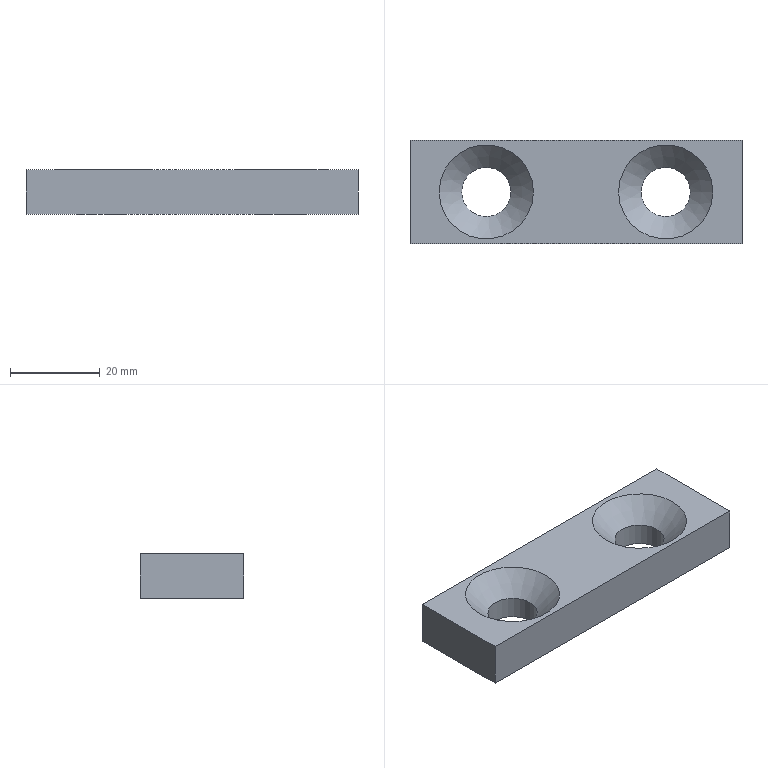Part | NX | features DATUM_CSYS 3, CSUNK_HOLE 2, HOLE PACKAGE 2, SKETCH 2, EXTRUDE 1, MIRROR_SET 1 | 1 solid | 10 faces | box 74 x 23 x 10 mm | volume 13994 mm3 | plane 6 | cylinder 2 | cone 2 | commonest cylinder face diameters 11 x2
STEP:
#1=CARTESIAN_POINT('',(-37.,-11.5,0.));
#2=VERTEX_POINT('',#1);
#3=CARTESIAN_POINT('',(37.,-11.5,0.));
#4=VERTEX_POINT('',#3);
#5=CARTESIAN_POINT('',(-37.,-11.5,0.));
#6=DIRECTION('',(1.,0.,0.));
#7=VECTOR('',#6,1000.);
#8=LINE('',#5,#7);
#9=EDGE_CURVE('',#2,#4,#8,.T.);
#10=ORIENTED_EDGE('',*,*,#9,.T.);
#11=CARTESIAN_POINT('',(37.,-11.5,10.));
#12=VERTEX_POINT('',#11);
#13=CARTESIAN_POINT('',(37.,-11.5,10.));
#14=DIRECTION('',(0.,0.,-1.));
#15=VECTOR('',#14,1000.);
#16=LINE('',#13,#15);
#17=EDGE_CURVE('',#12,#4,#16,.T.);
#18=ORIENTED_EDGE('',*,*,#17,.F.);
#19=CARTESIAN_POINT('',(-37.,-11.5,10.));
#20=VERTEX_POINT('',#19);
#21=CARTESIAN_POINT('',(-37.,-11.5,10.));
#22=DIRECTION('',(1.,0.,0.));
#23=VECTOR('',#22,1000.);
#24=LINE('',#21,#23);
#25=EDGE_CURVE('',#20,#12,#24,.T.);
#26=ORIENTED_EDGE('',*,*,#25,.F.);
#27=CARTESIAN_POINT('',(-37.,-11.5,10.));
#28=DIRECTION('',(0.,0.,-1.));
#29=VECTOR('',#28,1000.);
#30=LINE('',#27,#29);
#31=EDGE_CURVE('',#20,#2,#30,.T.);
#32=ORIENTED_EDGE('',*,*,#31,.T.);
#33=EDGE_LOOP('',(#10,#18,#26,#32));
#34=FACE_BOUND('',#33,.T.);
#35=CARTESIAN_POINT('',(-37.,-11.5,10.));
#36=DIRECTION('',(0.,1.,0.));
#37=DIRECTION('',(-1.,0.,0.));
#38=AXIS2_PLACEMENT_3D('',#35,#36,#37);
#39=PLANE('',#38);
#40=ADVANCED_FACE('',(#34),#39,.F.);
#41=CARTESIAN_POINT('',(37.,11.5,0.));
#42=VERTEX_POINT('',#41);
#43=CARTESIAN_POINT('',(37.,-11.5,0.));
#44=DIRECTION('',(0.,1.,0.));
#45=VECTOR('',#44,1000.);
#46=LINE('',#43,#45);
#47=EDGE_CURVE('',#4,#42,#46,.T.);
#48=ORIENTED_EDGE('',*,*,#47,.T.);
#49=CARTESIAN_POINT('',(37.,11.5,10.));
#50=VERTEX_POINT('',#49);
#51=CARTESIAN_POINT('',(37.,11.5,10.));
#52=DIRECTION('',(0.,0.,-1.));
#53=VECTOR('',#52,1000.);
#54=LINE('',#51,#53);
#55=EDGE_CURVE('',#50,#42,#54,.T.);
#56=ORIENTED_EDGE('',*,*,#55,.F.);
#57=CARTESIAN_POINT('',(37.,-11.5,10.));
#58=DIRECTION('',(0.,1.,0.));
#59=VECTOR('',#58,1000.);
#60=LINE('',#57,#59);
#61=EDGE_CURVE('',#12,#50,#60,.T.);
#62=ORIENTED_EDGE('',*,*,#61,.F.);
#63=ORIENTED_EDGE('',*,*,#17,.T.);
#64=EDGE_LOOP('',(#48,#56,#62,#63));
#65=FACE_BOUND('',#64,.T.);
#66=CARTESIAN_POINT('',(37.,-11.5,10.));
#67=DIRECTION('',(-1.,0.,0.));
#68=DIRECTION('',(0.,0.,1.));
#69=AXIS2_PLACEMENT_3D('',#66,#67,#68);
#70=PLANE('',#69);
#71=ADVANCED_FACE('',(#65),#70,.F.);
#72=CARTESIAN_POINT('',(-37.,11.5,0.));
#73=VERTEX_POINT('',#72);
#74=CARTESIAN_POINT('',(37.,11.5,0.));
#75=DIRECTION('',(-1.,0.,0.));
#76=VECTOR('',#75,1000.);
#77=LINE('',#74,#76);
#78=EDGE_CURVE('',#42,#73,#77,.T.);
#79=ORIENTED_EDGE('',*,*,#78,.T.);
#80=CARTESIAN_POINT('',(-37.,11.5,10.));
#81=VERTEX_POINT('',#80);
#82=CARTESIAN_POINT('',(-37.,11.5,10.));
#83=DIRECTION('',(0.,0.,-1.));
#84=VECTOR('',#83,1000.);
#85=LINE('',#82,#84);
#86=EDGE_CURVE('',#81,#73,#85,.T.);
#87=ORIENTED_EDGE('',*,*,#86,.F.);
#88=CARTESIAN_POINT('',(37.,11.5,10.));
#89=DIRECTION('',(-1.,0.,0.));
#90=VECTOR('',#89,1000.);
#91=LINE('',#88,#90);
#92=EDGE_CURVE('',#50,#81,#91,.T.);
#93=ORIENTED_EDGE('',*,*,#92,.F.);
#94=ORIENTED_EDGE('',*,*,#55,.T.);
#95=EDGE_LOOP('',(#79,#87,#93,#94));
#96=FACE_BOUND('',#95,.T.);
#97=CARTESIAN_POINT('',(37.,11.5,10.));
#98=DIRECTION('',(0.,-1.,0.));
#99=DIRECTION('',(1.,0.,0.));
#100=AXIS2_PLACEMENT_3D('',#97,#98,#99);
#101=PLANE('',#100);
#102=ADVANCED_FACE('',(#96),#101,.F.);
#103=CARTESIAN_POINT('',(-37.,11.5,0.));
#104=DIRECTION('',(0.,-1.,0.));
#105=VECTOR('',#104,1000.);
#106=LINE('',#103,#105);
#107=EDGE_CURVE('',#73,#2,#106,.T.);
#108=ORIENTED_EDGE('',*,*,#107,.T.);
#109=ORIENTED_EDGE('',*,*,#31,.F.);
#110=CARTESIAN_POINT('',(-37.,11.5,10.));
#111=DIRECTION('',(0.,-1.,0.));
#112=VECTOR('',#111,1000.);
#113=LINE('',#110,#112);
#114=EDGE_CURVE('',#81,#20,#113,.T.);
#115=ORIENTED_EDGE('',*,*,#114,.F.);
#116=ORIENTED_EDGE('',*,*,#86,.T.);
#117=EDGE_LOOP('',(#108,#109,#115,#116));
#118=FACE_BOUND('',#117,.T.);
#119=CARTESIAN_POINT('',(-37.,11.5,10.));
#120=DIRECTION('',(1.,0.,0.));
#121=DIRECTION('',(0.,0.,-1.));
#122=AXIS2_PLACEMENT_3D('',#119,#120,#121);
#123=PLANE('',#122);
#124=ADVANCED_FACE('',(#118),#123,.F.);
#125=CARTESIAN_POINT('',(30.5,0.,10.));
#126=VERTEX_POINT('',#125);
#127=CARTESIAN_POINT('',(20.,0.,10.));
#128=DIRECTION('',(0.,0.,1.));
#129=DIRECTION('',(1.,0.,0.));
#130=AXIS2_PLACEMENT_3D('',#127,#128,#129);
#131=CIRCLE('',#130,10.5);
#132=EDGE_CURVE('',#126,#126,#131,.T.);
#133=ORIENTED_EDGE('',*,*,#132,.F.);
#134=EDGE_LOOP('',(#133));
#135=FACE_BOUND('',#134,.T.);
#136=CARTESIAN_POINT('',(-30.5,0.,10.));
#137=VERTEX_POINT('',#136);
#138=CARTESIAN_POINT('',(-20.,0.,10.));
#139=DIRECTION('',(0.,0.,-1.));
#140=DIRECTION('',(-1.,0.,0.));
#141=AXIS2_PLACEMENT_3D('',#138,#139,#140);
#142=CIRCLE('',#141,10.5);
#143=EDGE_CURVE('',#137,#137,#142,.T.);
#144=ORIENTED_EDGE('',*,*,#143,.T.);
#145=EDGE_LOOP('',(#144));
#146=FACE_BOUND('',#145,.T.);
#147=ORIENTED_EDGE('',*,*,#25,.T.);
#148=ORIENTED_EDGE('',*,*,#61,.T.);
#149=ORIENTED_EDGE('',*,*,#92,.T.);
#150=ORIENTED_EDGE('',*,*,#114,.T.);
#151=EDGE_LOOP('',(#147,#148,#149,#150));
#152=FACE_BOUND('',#151,.T.);
#153=CARTESIAN_POINT('',(0.,0.,10.));
#154=DIRECTION('',(0.,0.,1.));
#155=DIRECTION('',(1.,0.,0.));
#156=AXIS2_PLACEMENT_3D('',#153,#154,#155);
#157=PLANE('',#156);
#158=ADVANCED_FACE('',(#135,#146,#152),#157,.T.);
#159=CARTESIAN_POINT('',(25.5,0.,0.));
#160=VERTEX_POINT('',#159);
#161=CARTESIAN_POINT('',(20.,0.,0.));
#162=DIRECTION('',(0.,0.,1.));
#163=DIRECTION('',(1.,0.,0.));
#164=AXIS2_PLACEMENT_3D('',#161,#162,#163);
#165=CIRCLE('',#164,5.5);
#166=EDGE_CURVE('',#160,#160,#165,.T.);
#167=ORIENTED_EDGE('',*,*,#166,.T.);
#168=EDGE_LOOP('',(#167));
#169=FACE_BOUND('',#168,.T.);
#170=CARTESIAN_POINT('',(-14.5,0.,0.));
#171=VERTEX_POINT('',#170);
#172=CARTESIAN_POINT('',(-20.,0.,0.));
#173=DIRECTION('',(0.,0.,1.));
#174=DIRECTION('',(1.,0.,0.));
#175=AXIS2_PLACEMENT_3D('',#172,#173,#174);
#176=CIRCLE('',#175,5.5);
#177=EDGE_CURVE('',#171,#171,#176,.T.);
#178=ORIENTED_EDGE('',*,*,#177,.T.);
#179=EDGE_LOOP('',(#178));
#180=FACE_BOUND('',#179,.T.);
#181=ORIENTED_EDGE('',*,*,#9,.F.);
#182=ORIENTED_EDGE('',*,*,#107,.F.);
#183=ORIENTED_EDGE('',*,*,#78,.F.);
#184=ORIENTED_EDGE('',*,*,#47,.F.);
#185=EDGE_LOOP('',(#181,#182,#183,#184));
#186=FACE_BOUND('',#185,.T.);
#187=CARTESIAN_POINT('',(0.,0.,0.));
#188=DIRECTION('',(0.,0.,1.));
#189=DIRECTION('',(1.,0.,0.));
#190=AXIS2_PLACEMENT_3D('',#187,#188,#189);
#191=PLANE('',#190);
#192=ADVANCED_FACE('',(#169,#180,#186),#191,.F.);
#193=CARTESIAN_POINT('',(-25.5,0.,5.));
#194=VERTEX_POINT('',#193);
#195=CARTESIAN_POINT('',(-20.,0.,5.));
#196=DIRECTION('',(0.,0.,-1.));
#197=DIRECTION('',(-1.,0.,0.));
#198=AXIS2_PLACEMENT_3D('',#195,#196,#197);
#199=CIRCLE('',#198,5.5);
#200=EDGE_CURVE('',#194,#194,#199,.F.);
#201=ORIENTED_EDGE('',*,*,#200,.T.);
#202=EDGE_LOOP('',(#201));
#203=FACE_BOUND('',#202,.T.);
#204=ORIENTED_EDGE('',*,*,#177,.F.);
#205=EDGE_LOOP('',(#204));
#206=FACE_BOUND('',#205,.T.);
#207=CARTESIAN_POINT('',(-20.,0.,-40.));
#208=DIRECTION('',(0.,0.,-1.));
#209=DIRECTION('',(-1.,0.,0.));
#210=AXIS2_PLACEMENT_3D('',#207,#208,#209);
#211=CYLINDRICAL_SURFACE('',#210,5.5);
#212=ADVANCED_FACE('',(#203,#206),#211,.F.);
#213=ORIENTED_EDGE('',*,*,#200,.F.);
#214=EDGE_LOOP('',(#213));
#215=FACE_BOUND('',#214,.T.);
#216=ORIENTED_EDGE('',*,*,#143,.F.);
#217=EDGE_LOOP('',(#216));
#218=FACE_BOUND('',#217,.T.);
#219=CARTESIAN_POINT('',(-20.,0.,10.));
#220=DIRECTION('',(0.,0.,1.));
#221=DIRECTION('',(1.,0.,0.));
#222=AXIS2_PLACEMENT_3D('',#219,#220,#221);
#223=CONICAL_SURFACE('',#222,10.5,0.7854);
#224=ADVANCED_FACE('',(#215,#218),#223,.F.);
#225=CARTESIAN_POINT('',(25.5,0.,5.));
#226=VERTEX_POINT('',#225);
#227=CARTESIAN_POINT('',(20.,0.,5.));
#228=DIRECTION('',(0.,0.,1.));
#229=DIRECTION('',(1.,0.,0.));
#230=AXIS2_PLACEMENT_3D('',#227,#228,#229);
#231=CIRCLE('',#230,5.5);
#232=EDGE_CURVE('',#226,#226,#231,.F.);
#233=ORIENTED_EDGE('',*,*,#232,.F.);
#234=EDGE_LOOP('',(#233));
#235=FACE_BOUND('',#234,.T.);
#236=ORIENTED_EDGE('',*,*,#166,.F.);
#237=EDGE_LOOP('',(#236));
#238=FACE_BOUND('',#237,.T.);
#239=CARTESIAN_POINT('',(20.,0.,-40.));
#240=DIRECTION('',(0.,0.,-1.));
#241=DIRECTION('',(1.,0.,0.));
#242=AXIS2_PLACEMENT_3D('',#239,#240,#241);
#243=CYLINDRICAL_SURFACE('',#242,5.5);
#244=ADVANCED_FACE('',(#235,#238),#243,.F.);
#245=ORIENTED_EDGE('',*,*,#232,.T.);
#246=EDGE_LOOP('',(#245));
#247=FACE_BOUND('',#246,.T.);
#248=ORIENTED_EDGE('',*,*,#132,.T.);
#249=EDGE_LOOP('',(#248));
#250=FACE_BOUND('',#249,.T.);
#251=CARTESIAN_POINT('',(20.,0.,10.));
#252=DIRECTION('',(0.,0.,1.));
#253=DIRECTION('',(-1.,0.,0.));
#254=AXIS2_PLACEMENT_3D('',#251,#252,#253);
#255=CONICAL_SURFACE('',#254,10.5,0.7854);
#256=ADVANCED_FACE('',(#247,#250),#255,.F.);
#257=CLOSED_SHELL('',(#40,#71,#102,#124,#158,#192,#212,#224,#244,#256));
#258=MANIFOLD_SOLID_BREP('',#257);
#259=(LENGTH_UNIT()NAMED_UNIT(*)SI_UNIT(.MILLI.,.METRE.));
#260=UNCERTAINTY_MEASURE_WITH_UNIT(LENGTH_MEASURE(0.00001),#259,'','');
#261=(NAMED_UNIT(*)PLANE_ANGLE_UNIT()SI_UNIT($,.RADIAN.));
#262=(NAMED_UNIT(*)SI_UNIT($,.STERADIAN.)SOLID_ANGLE_UNIT());
#263=(GEOMETRIC_REPRESENTATION_CONTEXT(3)GLOBAL_UNCERTAINTY_ASSIGNED_CONTEXT((#260))GLOBAL_UNIT_ASSIGNED_CONTEXT((#259,#261,#262))REPRESENTATION_CONTEXT('',''));
#264=ADVANCED_BREP_SHAPE_REPRESENTATION('',(#258),#263);